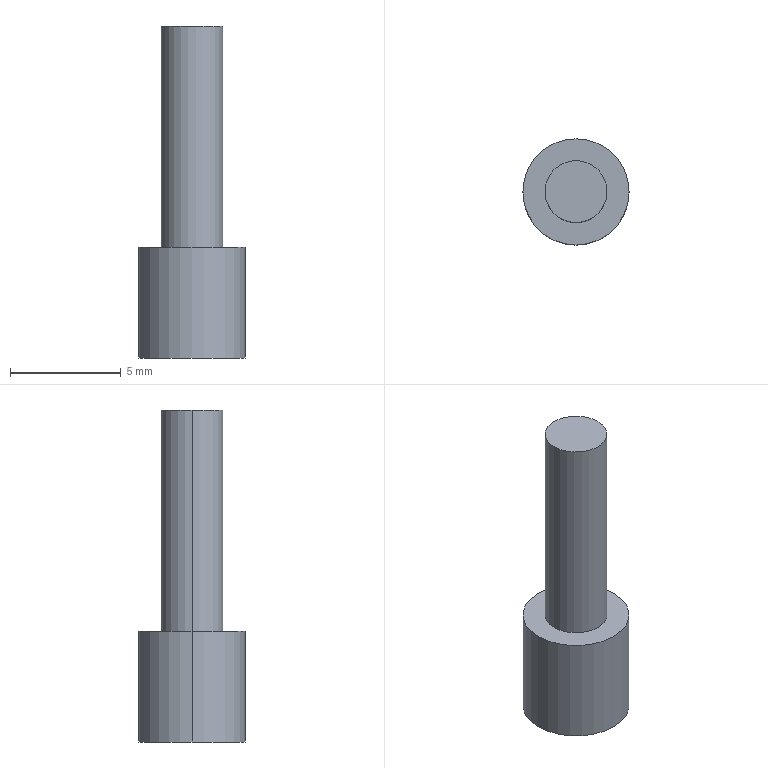Part | NX | 1 solid | 7 faces | box 4.8 x 4.8 x 15 mm | volume 152.053 mm3 | cylinder 4 | plane 3 | commonest cylinder face diameters 2.8 x2 4.8 x2
STEP:
#1=CARTESIAN_POINT('',(2.4,0.,-5.));
#2=VERTEX_POINT('',#1);
#3=CARTESIAN_POINT('',(-2.4,0.,-5.));
#4=VERTEX_POINT('',#3);
#5=CARTESIAN_POINT('',(0.,0.,-5.));
#6=DIRECTION('',(0.,0.,-1.));
#7=DIRECTION('',(-1.,0.,0.));
#8=AXIS2_PLACEMENT_3D('',#5,#6,#7);
#9=CIRCLE('',#8,2.4);
#10=EDGE_CURVE('',#2,#4,#9,.T.);
#11=ORIENTED_EDGE('',*,*,#10,.F.);
#12=CARTESIAN_POINT('',(2.4,0.,0.));
#13=VERTEX_POINT('',#12);
#14=CARTESIAN_POINT('',(2.4,0.,-5.));
#15=DIRECTION('',(0.,0.,1.));
#16=VECTOR('',#15,1000.);
#17=LINE('',#14,#16);
#18=EDGE_CURVE('',#2,#13,#17,.T.);
#19=ORIENTED_EDGE('',*,*,#18,.T.);
#20=CARTESIAN_POINT('',(-2.4,0.,0.));
#21=VERTEX_POINT('',#20);
#22=CARTESIAN_POINT('',(0.,0.,0.));
#23=DIRECTION('',(0.,0.,-1.));
#24=DIRECTION('',(-1.,0.,0.));
#25=AXIS2_PLACEMENT_3D('',#22,#23,#24);
#26=CIRCLE('',#25,2.4);
#27=EDGE_CURVE('',#13,#21,#26,.T.);
#28=ORIENTED_EDGE('',*,*,#27,.T.);
#29=CARTESIAN_POINT('',(-2.4,0.,-5.));
#30=DIRECTION('',(0.,0.,1.));
#31=VECTOR('',#30,1000.);
#32=LINE('',#29,#31);
#33=EDGE_CURVE('',#4,#21,#32,.T.);
#34=ORIENTED_EDGE('',*,*,#33,.F.);
#35=EDGE_LOOP('',(#11,#19,#28,#34));
#36=FACE_BOUND('',#35,.T.);
#37=CARTESIAN_POINT('',(0.,0.,-5.));
#38=DIRECTION('',(0.,0.,1.));
#39=DIRECTION('',(1.,0.,0.));
#40=AXIS2_PLACEMENT_3D('',#37,#38,#39);
#41=CYLINDRICAL_SURFACE('',#40,2.4);
#42=ADVANCED_FACE('',(#36),#41,.T.);
#43=CARTESIAN_POINT('',(1.4,0.,0.));
#44=VERTEX_POINT('',#43);
#45=CARTESIAN_POINT('',(-1.4,0.,0.));
#46=VERTEX_POINT('',#45);
#47=CARTESIAN_POINT('',(0.,0.,0.));
#48=DIRECTION('',(0.,0.,-1.));
#49=DIRECTION('',(-1.,0.,0.));
#50=AXIS2_PLACEMENT_3D('',#47,#48,#49);
#51=CIRCLE('',#50,1.4);
#52=EDGE_CURVE('',#44,#46,#51,.T.);
#53=ORIENTED_EDGE('',*,*,#52,.F.);
#54=CARTESIAN_POINT('',(1.4,0.,10.));
#55=VERTEX_POINT('',#54);
#56=CARTESIAN_POINT('',(1.4,0.,10.));
#57=DIRECTION('',(0.,0.,-1.));
#58=VECTOR('',#57,1000.);
#59=LINE('',#56,#58);
#60=EDGE_CURVE('',#44,#55,#59,.F.);
#61=ORIENTED_EDGE('',*,*,#60,.T.);
#62=CARTESIAN_POINT('',(-1.4,0.,10.));
#63=VERTEX_POINT('',#62);
#64=CARTESIAN_POINT('',(0.,0.,10.));
#65=DIRECTION('',(0.,0.,1.));
#66=DIRECTION('',(1.,0.,0.));
#67=AXIS2_PLACEMENT_3D('',#64,#65,#66);
#68=CIRCLE('',#67,1.4);
#69=EDGE_CURVE('',#63,#55,#68,.T.);
#70=ORIENTED_EDGE('',*,*,#69,.F.);
#71=CARTESIAN_POINT('',(-1.4,0.,10.));
#72=DIRECTION('',(0.,0.,-1.));
#73=VECTOR('',#72,1000.);
#74=LINE('',#71,#73);
#75=EDGE_CURVE('',#46,#63,#74,.F.);
#76=ORIENTED_EDGE('',*,*,#75,.F.);
#77=EDGE_LOOP('',(#53,#61,#70,#76));
#78=FACE_BOUND('',#77,.T.);
#79=CARTESIAN_POINT('',(0.,0.,10.));
#80=DIRECTION('',(0.,0.,-1.));
#81=DIRECTION('',(-1.,0.,0.));
#82=AXIS2_PLACEMENT_3D('',#79,#80,#81);
#83=CYLINDRICAL_SURFACE('',#82,1.4);
#84=ADVANCED_FACE('',(#78),#83,.T.);
#85=ORIENTED_EDGE('',*,*,#10,.T.);
#86=CARTESIAN_POINT('',(0.,0.,-5.));
#87=DIRECTION('',(0.,0.,-1.));
#88=DIRECTION('',(-1.,0.,0.));
#89=AXIS2_PLACEMENT_3D('',#86,#87,#88);
#90=CIRCLE('',#89,2.4);
#91=EDGE_CURVE('',#4,#2,#90,.T.);
#92=ORIENTED_EDGE('',*,*,#91,.T.);
#93=EDGE_LOOP('',(#85,#92));
#94=FACE_BOUND('',#93,.T.);
#95=CARTESIAN_POINT('',(0.,0.,-5.));
#96=DIRECTION('',(0.,0.,-1.));
#97=DIRECTION('',(0.,-1.,0.));
#98=AXIS2_PLACEMENT_3D('',#95,#96,#97);
#99=PLANE('',#98);
#100=ADVANCED_FACE('',(#94),#99,.T.);
#101=ORIENTED_EDGE('',*,*,#69,.T.);
#102=CARTESIAN_POINT('',(0.,0.,10.));
#103=DIRECTION('',(0.,0.,1.));
#104=DIRECTION('',(1.,0.,0.));
#105=AXIS2_PLACEMENT_3D('',#102,#103,#104);
#106=CIRCLE('',#105,1.4);
#107=EDGE_CURVE('',#55,#63,#106,.T.);
#108=ORIENTED_EDGE('',*,*,#107,.T.);
#109=EDGE_LOOP('',(#101,#108));
#110=FACE_BOUND('',#109,.T.);
#111=CARTESIAN_POINT('',(0.,0.,10.));
#112=DIRECTION('',(0.,0.,1.));
#113=DIRECTION('',(1.,0.,0.));
#114=AXIS2_PLACEMENT_3D('',#111,#112,#113);
#115=PLANE('',#114);
#116=ADVANCED_FACE('',(#110),#115,.T.);
#117=ORIENTED_EDGE('',*,*,#27,.F.);
#118=CARTESIAN_POINT('',(0.,0.,0.));
#119=DIRECTION('',(0.,0.,-1.));
#120=DIRECTION('',(-1.,0.,0.));
#121=AXIS2_PLACEMENT_3D('',#118,#119,#120);
#122=CIRCLE('',#121,2.4);
#123=EDGE_CURVE('',#21,#13,#122,.T.);
#124=ORIENTED_EDGE('',*,*,#123,.F.);
#125=EDGE_LOOP('',(#117,#124));
#126=FACE_BOUND('',#125,.T.);
#127=ORIENTED_EDGE('',*,*,#52,.T.);
#128=CARTESIAN_POINT('',(0.,0.,0.));
#129=DIRECTION('',(0.,0.,-1.));
#130=DIRECTION('',(-1.,0.,0.));
#131=AXIS2_PLACEMENT_3D('',#128,#129,#130);
#132=CIRCLE('',#131,1.4);
#133=EDGE_CURVE('',#46,#44,#132,.T.);
#134=ORIENTED_EDGE('',*,*,#133,.T.);
#135=EDGE_LOOP('',(#127,#134));
#136=FACE_BOUND('',#135,.T.);
#137=CARTESIAN_POINT('',(0.,0.,0.));
#138=DIRECTION('',(0.,0.,-1.));
#139=DIRECTION('',(0.,-1.,0.));
#140=AXIS2_PLACEMENT_3D('',#137,#138,#139);
#141=PLANE('',#140);
#142=ADVANCED_FACE('',(#126,#136),#141,.F.);
#143=ORIENTED_EDGE('',*,*,#75,.T.);
#144=ORIENTED_EDGE('',*,*,#107,.F.);
#145=ORIENTED_EDGE('',*,*,#60,.F.);
#146=ORIENTED_EDGE('',*,*,#133,.F.);
#147=EDGE_LOOP('',(#143,#144,#145,#146));
#148=FACE_BOUND('',#147,.T.);
#149=CARTESIAN_POINT('',(0.,0.,10.));
#150=DIRECTION('',(0.,0.,-1.));
#151=DIRECTION('',(-1.,0.,0.));
#152=AXIS2_PLACEMENT_3D('',#149,#150,#151);
#153=CYLINDRICAL_SURFACE('',#152,1.4);
#154=ADVANCED_FACE('',(#148),#153,.T.);
#155=ORIENTED_EDGE('',*,*,#18,.F.);
#156=ORIENTED_EDGE('',*,*,#91,.F.);
#157=ORIENTED_EDGE('',*,*,#33,.T.);
#158=ORIENTED_EDGE('',*,*,#123,.T.);
#159=EDGE_LOOP('',(#155,#156,#157,#158));
#160=FACE_BOUND('',#159,.T.);
#161=CARTESIAN_POINT('',(0.,0.,-5.));
#162=DIRECTION('',(0.,0.,1.));
#163=DIRECTION('',(1.,0.,0.));
#164=AXIS2_PLACEMENT_3D('',#161,#162,#163);
#165=CYLINDRICAL_SURFACE('',#164,2.4);
#166=ADVANCED_FACE('',(#160),#165,.T.);
#167=CLOSED_SHELL('',(#42,#84,#100,#116,#142,#154,#166));
#168=MANIFOLD_SOLID_BREP('',#167);
#169=(LENGTH_UNIT()NAMED_UNIT(*)SI_UNIT(.MILLI.,.METRE.));
#170=UNCERTAINTY_MEASURE_WITH_UNIT(LENGTH_MEASURE(0.00001),#169,'','');
#171=(NAMED_UNIT(*)PLANE_ANGLE_UNIT()SI_UNIT($,.RADIAN.));
#172=(NAMED_UNIT(*)SI_UNIT($,.STERADIAN.)SOLID_ANGLE_UNIT());
#173=(GEOMETRIC_REPRESENTATION_CONTEXT(3)GLOBAL_UNCERTAINTY_ASSIGNED_CONTEXT((#170))GLOBAL_UNIT_ASSIGNED_CONTEXT((#169,#171,#172))REPRESENTATION_CONTEXT('',''));
#174=ADVANCED_BREP_SHAPE_REPRESENTATION('',(#168),#173);